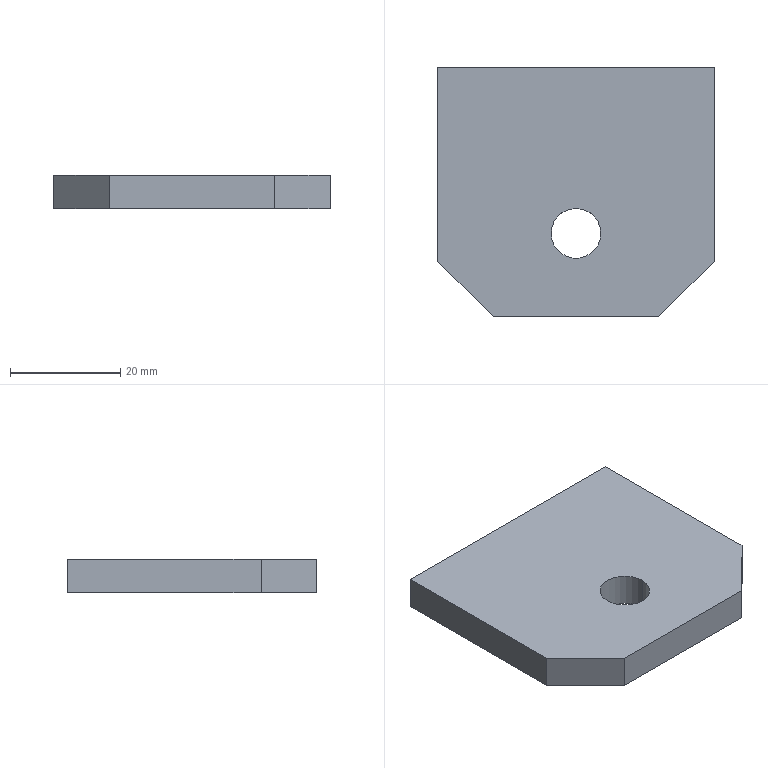Part | SolidWorks | features Chamfer 1, Cut 1, Extrusion 1 | 1 solid | 10 faces | box 50 x 45 x 6 mm | volume 12518 mm3 | plane 8 | cylinder 2 | commonest cylinder face diameters 9 x2
STEP:
#1=CARTESIAN_POINT('',(-4.5,-7.5,0.));
#2=VERTEX_POINT('',#1);
#3=CARTESIAN_POINT('',(4.5,-7.5,0.));
#4=VERTEX_POINT('',#3);
#5=CARTESIAN_POINT('',(0.,-7.5,0.));
#6=DIRECTION('',(0.,0.,1.));
#7=DIRECTION('',(1.,0.,0.));
#8=AXIS2_PLACEMENT_3D('',#5,#6,#7);
#9=CIRCLE('',#8,4.5);
#10=EDGE_CURVE('',#2,#4,#9,.T.);
#11=ORIENTED_EDGE('',*,*,#10,.F.);
#12=CARTESIAN_POINT('',(-4.5,-7.5,6.));
#13=VERTEX_POINT('',#12);
#14=CARTESIAN_POINT('',(-4.5,-7.5,0.));
#15=DIRECTION('',(0.,0.,1.));
#16=VECTOR('',#15,1000.);
#17=LINE('',#14,#16);
#18=EDGE_CURVE('',#2,#13,#17,.T.);
#19=ORIENTED_EDGE('',*,*,#18,.T.);
#20=CARTESIAN_POINT('',(4.5,-7.5,6.));
#21=VERTEX_POINT('',#20);
#22=CARTESIAN_POINT('',(0.,-7.5,6.));
#23=DIRECTION('',(0.,0.,1.));
#24=DIRECTION('',(1.,0.,0.));
#25=AXIS2_PLACEMENT_3D('',#22,#23,#24);
#26=CIRCLE('',#25,4.5);
#27=EDGE_CURVE('',#13,#21,#26,.T.);
#28=ORIENTED_EDGE('',*,*,#27,.T.);
#29=CARTESIAN_POINT('',(4.5,-7.5,0.));
#30=DIRECTION('',(0.,0.,1.));
#31=VECTOR('',#30,1000.);
#32=LINE('',#29,#31);
#33=EDGE_CURVE('',#4,#21,#32,.T.);
#34=ORIENTED_EDGE('',*,*,#33,.F.);
#35=EDGE_LOOP('',(#11,#19,#28,#34));
#36=FACE_OUTER_BOUND('',#35,.T.);
#37=CARTESIAN_POINT('',(0.,-7.5,0.));
#38=DIRECTION('',(0.,0.,1.));
#39=DIRECTION('',(1.,0.,0.));
#40=AXIS2_PLACEMENT_3D('',#37,#38,#39);
#41=CYLINDRICAL_SURFACE('',#40,4.5);
#42=ADVANCED_FACE('',(#36),#41,.F.);
#43=CARTESIAN_POINT('',(25.,-12.5,6.));
#44=VERTEX_POINT('',#43);
#45=CARTESIAN_POINT('',(25.,22.5,6.));
#46=VERTEX_POINT('',#45);
#47=CARTESIAN_POINT('',(25.,-22.5,6.));
#48=DIRECTION('',(0.,1.,0.));
#49=VECTOR('',#48,1000.);
#50=LINE('',#47,#49);
#51=EDGE_CURVE('',#44,#46,#50,.T.);
#52=ORIENTED_EDGE('',*,*,#51,.F.);
#53=CARTESIAN_POINT('',(25.,-12.5,0.));
#54=VERTEX_POINT('',#53);
#55=CARTESIAN_POINT('',(25.,-12.5,6.));
#56=DIRECTION('',(0.,0.,-1.));
#57=VECTOR('',#56,1000.);
#58=LINE('',#55,#57);
#59=EDGE_CURVE('',#44,#54,#58,.T.);
#60=ORIENTED_EDGE('',*,*,#59,.T.);
#61=CARTESIAN_POINT('',(25.,22.5,0.));
#62=VERTEX_POINT('',#61);
#63=CARTESIAN_POINT('',(25.,-22.5,0.));
#64=DIRECTION('',(0.,1.,0.));
#65=VECTOR('',#64,1000.);
#66=LINE('',#63,#65);
#67=EDGE_CURVE('',#54,#62,#66,.T.);
#68=ORIENTED_EDGE('',*,*,#67,.T.);
#69=CARTESIAN_POINT('',(25.,22.5,6.));
#70=DIRECTION('',(0.,0.,-1.));
#71=VECTOR('',#70,1000.);
#72=LINE('',#69,#71);
#73=EDGE_CURVE('',#46,#62,#72,.T.);
#74=ORIENTED_EDGE('',*,*,#73,.F.);
#75=EDGE_LOOP('',(#52,#60,#68,#74));
#76=FACE_OUTER_BOUND('',#75,.T.);
#77=CARTESIAN_POINT('',(25.,-22.5,6.));
#78=DIRECTION('',(-1.,0.,0.));
#79=DIRECTION('',(0.,0.,1.));
#80=AXIS2_PLACEMENT_3D('',#77,#78,#79);
#81=PLANE('',#80);
#82=ADVANCED_FACE('',(#76),#81,.F.);
#83=CARTESIAN_POINT('',(-25.,22.5,0.));
#84=VERTEX_POINT('',#83);
#85=CARTESIAN_POINT('',(-25.,22.5,0.));
#86=DIRECTION('',(-1.,0.,0.));
#87=VECTOR('',#86,1000.);
#88=LINE('',#85,#87);
#89=EDGE_CURVE('',#62,#84,#88,.T.);
#90=ORIENTED_EDGE('',*,*,#89,.T.);
#91=CARTESIAN_POINT('',(-25.,22.5,6.));
#92=VERTEX_POINT('',#91);
#93=CARTESIAN_POINT('',(-25.,22.5,6.));
#94=DIRECTION('',(0.,0.,-1.));
#95=VECTOR('',#94,1000.);
#96=LINE('',#93,#95);
#97=EDGE_CURVE('',#92,#84,#96,.T.);
#98=ORIENTED_EDGE('',*,*,#97,.F.);
#99=CARTESIAN_POINT('',(-25.,22.5,6.));
#100=DIRECTION('',(-1.,0.,0.));
#101=VECTOR('',#100,1000.);
#102=LINE('',#99,#101);
#103=EDGE_CURVE('',#46,#92,#102,.T.);
#104=ORIENTED_EDGE('',*,*,#103,.F.);
#105=ORIENTED_EDGE('',*,*,#73,.T.);
#106=EDGE_LOOP('',(#90,#98,#104,#105));
#107=FACE_OUTER_BOUND('',#106,.T.);
#108=CARTESIAN_POINT('',(-25.,22.5,6.));
#109=DIRECTION('',(0.,-1.,0.));
#110=DIRECTION('',(0.,0.,-1.));
#111=AXIS2_PLACEMENT_3D('',#108,#109,#110);
#112=PLANE('',#111);
#113=ADVANCED_FACE('',(#107),#112,.F.);
#114=CARTESIAN_POINT('',(-25.,-12.5,0.));
#115=VERTEX_POINT('',#114);
#116=CARTESIAN_POINT('',(-25.,-22.5,0.));
#117=DIRECTION('',(0.,-1.,0.));
#118=VECTOR('',#117,1000.);
#119=LINE('',#116,#118);
#120=EDGE_CURVE('',#84,#115,#119,.T.);
#121=ORIENTED_EDGE('',*,*,#120,.T.);
#122=CARTESIAN_POINT('',(-25.,-12.5,6.));
#123=VERTEX_POINT('',#122);
#124=CARTESIAN_POINT('',(-25.,-12.5,6.));
#125=DIRECTION('',(0.,0.,1.));
#126=VECTOR('',#125,1000.);
#127=LINE('',#124,#126);
#128=EDGE_CURVE('',#115,#123,#127,.T.);
#129=ORIENTED_EDGE('',*,*,#128,.T.);
#130=CARTESIAN_POINT('',(-25.,-22.5,6.));
#131=DIRECTION('',(0.,-1.,0.));
#132=VECTOR('',#131,1000.);
#133=LINE('',#130,#132);
#134=EDGE_CURVE('',#92,#123,#133,.T.);
#135=ORIENTED_EDGE('',*,*,#134,.F.);
#136=ORIENTED_EDGE('',*,*,#97,.T.);
#137=EDGE_LOOP('',(#121,#129,#135,#136));
#138=FACE_OUTER_BOUND('',#137,.T.);
#139=CARTESIAN_POINT('',(-25.,-22.5,6.));
#140=DIRECTION('',(1.,0.,0.));
#141=DIRECTION('',(0.,0.,-1.));
#142=AXIS2_PLACEMENT_3D('',#139,#140,#141);
#143=PLANE('',#142);
#144=ADVANCED_FACE('',(#138),#143,.F.);
#145=CARTESIAN_POINT('',(-15.,-22.5,6.));
#146=VERTEX_POINT('',#145);
#147=CARTESIAN_POINT('',(15.,-22.5,6.));
#148=VERTEX_POINT('',#147);
#149=CARTESIAN_POINT('',(-25.,-22.5,6.));
#150=DIRECTION('',(1.,0.,0.));
#151=VECTOR('',#150,1000.);
#152=LINE('',#149,#151);
#153=EDGE_CURVE('',#146,#148,#152,.T.);
#154=ORIENTED_EDGE('',*,*,#153,.F.);
#155=CARTESIAN_POINT('',(-15.,-22.5,0.));
#156=VERTEX_POINT('',#155);
#157=CARTESIAN_POINT('',(-15.,-22.5,6.));
#158=DIRECTION('',(0.,0.,-1.));
#159=VECTOR('',#158,1000.);
#160=LINE('',#157,#159);
#161=EDGE_CURVE('',#146,#156,#160,.T.);
#162=ORIENTED_EDGE('',*,*,#161,.T.);
#163=CARTESIAN_POINT('',(15.,-22.5,0.));
#164=VERTEX_POINT('',#163);
#165=CARTESIAN_POINT('',(-25.,-22.5,0.));
#166=DIRECTION('',(1.,0.,0.));
#167=VECTOR('',#166,1000.);
#168=LINE('',#165,#167);
#169=EDGE_CURVE('',#156,#164,#168,.T.);
#170=ORIENTED_EDGE('',*,*,#169,.T.);
#171=CARTESIAN_POINT('',(15.,-22.5,6.));
#172=DIRECTION('',(0.,0.,1.));
#173=VECTOR('',#172,1000.);
#174=LINE('',#171,#173);
#175=EDGE_CURVE('',#164,#148,#174,.T.);
#176=ORIENTED_EDGE('',*,*,#175,.T.);
#177=EDGE_LOOP('',(#154,#162,#170,#176));
#178=FACE_OUTER_BOUND('',#177,.T.);
#179=CARTESIAN_POINT('',(-25.,-22.5,6.));
#180=DIRECTION('',(0.,1.,0.));
#181=DIRECTION('',(0.,0.,1.));
#182=AXIS2_PLACEMENT_3D('',#179,#180,#181);
#183=PLANE('',#182);
#184=ADVANCED_FACE('',(#178),#183,.F.);
#185=CARTESIAN_POINT('',(0.,-7.5,6.));
#186=DIRECTION('',(0.,0.,1.));
#187=DIRECTION('',(1.,0.,0.));
#188=AXIS2_PLACEMENT_3D('',#185,#186,#187);
#189=CIRCLE('',#188,4.5);
#190=EDGE_CURVE('',#21,#13,#189,.T.);
#191=ORIENTED_EDGE('',*,*,#190,.F.);
#192=ORIENTED_EDGE('',*,*,#27,.F.);
#193=EDGE_LOOP('',(#191,#192));
#194=FACE_BOUND('',#193,.T.);
#195=ORIENTED_EDGE('',*,*,#134,.T.);
#196=CARTESIAN_POINT('',(-15.,-22.5,6.));
#197=DIRECTION('',(0.7071,-0.7071,0.));
#198=VECTOR('',#197,1000.);
#199=LINE('',#196,#198);
#200=EDGE_CURVE('',#123,#146,#199,.T.);
#201=ORIENTED_EDGE('',*,*,#200,.T.);
#202=ORIENTED_EDGE('',*,*,#153,.T.);
#203=CARTESIAN_POINT('',(25.,-12.5,6.));
#204=DIRECTION('',(0.7071,0.7071,0.));
#205=VECTOR('',#204,1000.);
#206=LINE('',#203,#205);
#207=EDGE_CURVE('',#148,#44,#206,.T.);
#208=ORIENTED_EDGE('',*,*,#207,.T.);
#209=ORIENTED_EDGE('',*,*,#51,.T.);
#210=ORIENTED_EDGE('',*,*,#103,.T.);
#211=EDGE_LOOP('',(#195,#201,#202,#208,#209,#210));
#212=FACE_OUTER_BOUND('',#211,.T.);
#213=CARTESIAN_POINT('',(0.,0.,6.));
#214=DIRECTION('',(0.,0.,-1.));
#215=DIRECTION('',(-1.,0.,0.));
#216=AXIS2_PLACEMENT_3D('',#213,#214,#215);
#217=PLANE('',#216);
#218=ADVANCED_FACE('',(#194,#212),#217,.F.);
#219=CARTESIAN_POINT('',(0.,-7.5,0.));
#220=DIRECTION('',(0.,0.,1.));
#221=DIRECTION('',(1.,0.,0.));
#222=AXIS2_PLACEMENT_3D('',#219,#220,#221);
#223=CIRCLE('',#222,4.5);
#224=EDGE_CURVE('',#4,#2,#223,.T.);
#225=ORIENTED_EDGE('',*,*,#224,.T.);
#226=ORIENTED_EDGE('',*,*,#10,.T.);
#227=EDGE_LOOP('',(#225,#226));
#228=FACE_BOUND('',#227,.T.);
#229=ORIENTED_EDGE('',*,*,#169,.F.);
#230=CARTESIAN_POINT('',(-18.75,-18.75,0.));
#231=DIRECTION('',(-0.7071,0.7071,0.));
#232=VECTOR('',#231,1000.);
#233=LINE('',#230,#232);
#234=EDGE_CURVE('',#156,#115,#233,.T.);
#235=ORIENTED_EDGE('',*,*,#234,.T.);
#236=ORIENTED_EDGE('',*,*,#120,.F.);
#237=ORIENTED_EDGE('',*,*,#89,.F.);
#238=ORIENTED_EDGE('',*,*,#67,.F.);
#239=CARTESIAN_POINT('',(18.75,-18.75,0.));
#240=DIRECTION('',(-0.7071,-0.7071,0.));
#241=VECTOR('',#240,1000.);
#242=LINE('',#239,#241);
#243=EDGE_CURVE('',#54,#164,#242,.T.);
#244=ORIENTED_EDGE('',*,*,#243,.T.);
#245=EDGE_LOOP('',(#229,#235,#236,#237,#238,#244));
#246=FACE_OUTER_BOUND('',#245,.T.);
#247=CARTESIAN_POINT('',(0.,0.,0.));
#248=DIRECTION('',(0.,0.,-1.));
#249=DIRECTION('',(-1.,0.,0.));
#250=AXIS2_PLACEMENT_3D('',#247,#248,#249);
#251=PLANE('',#250);
#252=ADVANCED_FACE('',(#228,#246),#251,.T.);
#253=ORIENTED_EDGE('',*,*,#18,.F.);
#254=ORIENTED_EDGE('',*,*,#224,.F.);
#255=ORIENTED_EDGE('',*,*,#33,.T.);
#256=ORIENTED_EDGE('',*,*,#190,.T.);
#257=EDGE_LOOP('',(#253,#254,#255,#256));
#258=FACE_OUTER_BOUND('',#257,.T.);
#259=CARTESIAN_POINT('',(0.,-7.5,0.));
#260=DIRECTION('',(0.,0.,1.));
#261=DIRECTION('',(1.,0.,0.));
#262=AXIS2_PLACEMENT_3D('',#259,#260,#261);
#263=CYLINDRICAL_SURFACE('',#262,4.5);
#264=ADVANCED_FACE('',(#258),#263,.F.);
#265=ORIENTED_EDGE('',*,*,#200,.F.);
#266=ORIENTED_EDGE('',*,*,#128,.F.);
#267=ORIENTED_EDGE('',*,*,#234,.F.);
#268=ORIENTED_EDGE('',*,*,#161,.F.);
#269=EDGE_LOOP('',(#265,#266,#267,#268));
#270=FACE_OUTER_BOUND('',#269,.T.);
#271=CARTESIAN_POINT('',(-15.,-22.5,6.));
#272=DIRECTION('',(0.7071,0.7071,0.));
#273=DIRECTION('',(0.,0.,-1.));
#274=AXIS2_PLACEMENT_3D('',#271,#272,#273);
#275=PLANE('',#274);
#276=ADVANCED_FACE('',(#270),#275,.F.);
#277=ORIENTED_EDGE('',*,*,#207,.F.);
#278=ORIENTED_EDGE('',*,*,#175,.F.);
#279=ORIENTED_EDGE('',*,*,#243,.F.);
#280=ORIENTED_EDGE('',*,*,#59,.F.);
#281=EDGE_LOOP('',(#277,#278,#279,#280));
#282=FACE_OUTER_BOUND('',#281,.T.);
#283=CARTESIAN_POINT('',(25.,-12.5,6.));
#284=DIRECTION('',(-0.7071,0.7071,0.));
#285=DIRECTION('',(0.,0.,-1.));
#286=AXIS2_PLACEMENT_3D('',#283,#284,#285);
#287=PLANE('',#286);
#288=ADVANCED_FACE('',(#282),#287,.F.);
#289=CLOSED_SHELL('',(#42,#82,#113,#144,#184,#218,#252,#264,#276,#288));
#290=MANIFOLD_SOLID_BREP('',#289);
#291=CARTESIAN_POINT('',(0.,0.,0.));
#292=DIRECTION('',(0.,0.,1.));
#293=DIRECTION('',(1.,0.,0.));
#294=AXIS2_PLACEMENT_3D('',#291,#292,#293);
#295=(LENGTH_UNIT()NAMED_UNIT(*)SI_UNIT(.MILLI.,.METRE.));
#296=UNCERTAINTY_MEASURE_WITH_UNIT(LENGTH_MEASURE(0.00001),#295,'','');
#297=(NAMED_UNIT(*)PLANE_ANGLE_UNIT()SI_UNIT($,.RADIAN.));
#298=(NAMED_UNIT(*)SI_UNIT($,.STERADIAN.)SOLID_ANGLE_UNIT());
#299=(GEOMETRIC_REPRESENTATION_CONTEXT(3)GLOBAL_UNCERTAINTY_ASSIGNED_CONTEXT((#296))GLOBAL_UNIT_ASSIGNED_CONTEXT((#295,#297,#298))REPRESENTATION_CONTEXT('',''));
#300=ADVANCED_BREP_SHAPE_REPRESENTATION('',(#290,#294),#299);